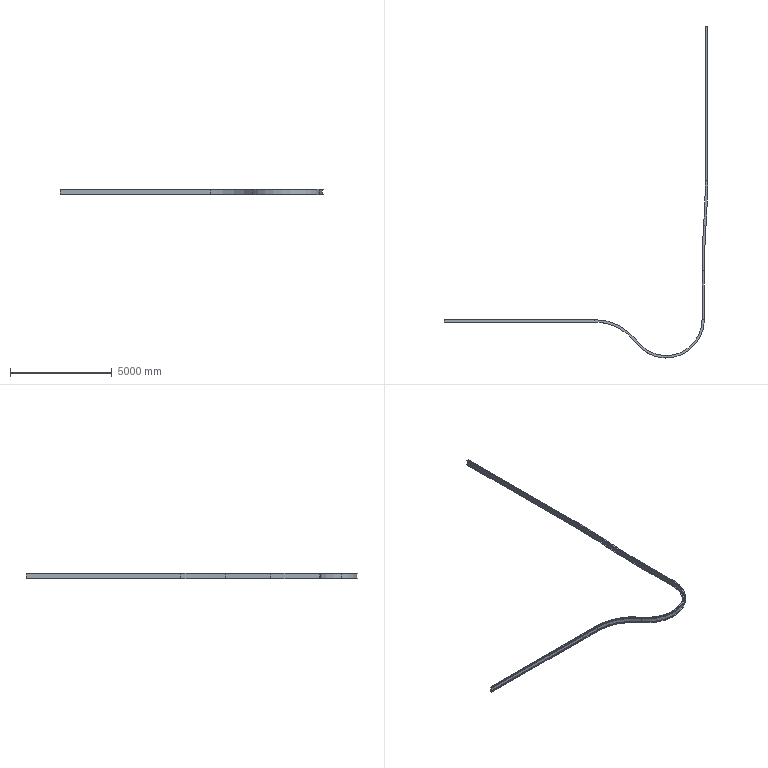Part | SolidWorks | features BaseBody 1 | 1 solid | 142 faces | box 12904 x 16279 x 250 mm | volume 148415394 mm3 | cylinder 48 | plane 46 | torus 32 | cone 16 | commonest cylinder face diameters 10 x12 20 x12 3522 x2 3758 x2 4942 x2 5178 x2